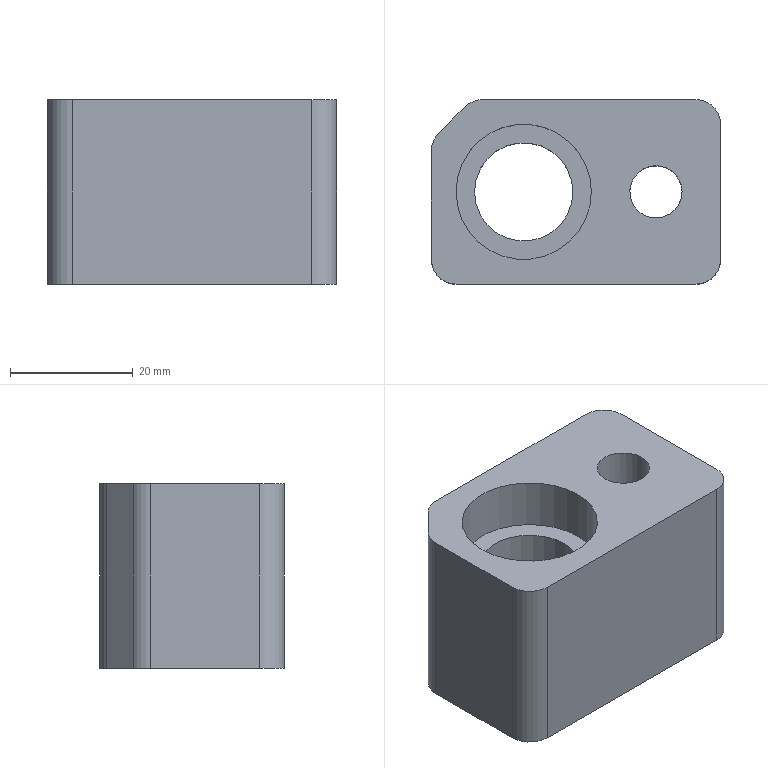Part | NX | features 7 2 | 1 solid | 18 faces | box 47 x 30 x 30 mm | volume 30463 mm3 | plane 9 | cylinder 9 | commonest cylinder face diameters 8 x5 8.5 x1 14.5 x1 16 x1 22 x1
STEP:
#1=CARTESIAN_POINT('',(3123.747,81.578,91.));
#2=VERTEX_POINT('',#1);
#3=CARTESIAN_POINT('',(3123.747,77.328,91.));
#4=DIRECTION('',(0.,0.,-1.));
#5=DIRECTION('',(0.,1.,0.));
#6=AXIS2_PLACEMENT_3D('',#3,#4,#5);
#7=CIRCLE('',#6,4.25);
#8=EDGE_CURVE('',#2,#2,#7,.T.);
#9=ORIENTED_EDGE('',*,*,#8,.T.);
#10=EDGE_LOOP('',(#9));
#11=FACE_BOUND('',#10,.T.);
#12=CARTESIAN_POINT('',(3130.247,62.328,91.));
#13=VERTEX_POINT('',#12);
#14=CARTESIAN_POINT('',(3091.247,62.328,91.));
#15=VERTEX_POINT('',#14);
#16=CARTESIAN_POINT('',(3102.247,62.328,91.));
#17=DIRECTION('',(-1.,0.,0.));
#18=VECTOR('',#17,1000.);
#19=LINE('',#16,#18);
#20=EDGE_CURVE('',#13,#15,#19,.T.);
#21=ORIENTED_EDGE('',*,*,#20,.F.);
#22=CARTESIAN_POINT('',(3134.247,66.328,91.));
#23=VERTEX_POINT('',#22);
#24=CARTESIAN_POINT('',(3130.247,66.328,91.));
#25=DIRECTION('',(0.,0.,1.));
#26=DIRECTION('',(0.,1.,0.));
#27=AXIS2_PLACEMENT_3D('',#24,#25,#26);
#28=CIRCLE('',#27,4.);
#29=EDGE_CURVE('',#13,#23,#28,.T.);
#30=ORIENTED_EDGE('',*,*,#29,.T.);
#31=CARTESIAN_POINT('',(3134.247,88.328,91.));
#32=VERTEX_POINT('',#31);
#33=CARTESIAN_POINT('',(3134.247,77.328,91.));
#34=DIRECTION('',(0.,-1.,0.));
#35=VECTOR('',#34,1000.);
#36=LINE('',#33,#35);
#37=EDGE_CURVE('',#32,#23,#36,.T.);
#38=ORIENTED_EDGE('',*,*,#37,.F.);
#39=CARTESIAN_POINT('',(3130.247,92.328,91.));
#40=VERTEX_POINT('',#39);
#41=CARTESIAN_POINT('',(3130.247,88.328,91.));
#42=DIRECTION('',(0.,0.,1.));
#43=DIRECTION('',(0.,1.,0.));
#44=AXIS2_PLACEMENT_3D('',#41,#42,#43);
#45=CIRCLE('',#44,4.);
#46=EDGE_CURVE('',#32,#40,#45,.T.);
#47=ORIENTED_EDGE('',*,*,#46,.T.);
#48=CARTESIAN_POINT('',(3095.54,92.328,91.));
#49=VERTEX_POINT('',#48);
#50=CARTESIAN_POINT('',(3102.247,92.328,91.));
#51=DIRECTION('',(1.,0.,0.));
#52=VECTOR('',#51,1000.);
#53=LINE('',#50,#52);
#54=EDGE_CURVE('',#49,#40,#53,.T.);
#55=ORIENTED_EDGE('',*,*,#54,.F.);
#56=CARTESIAN_POINT('',(3092.711,91.157,91.));
#57=VERTEX_POINT('',#56);
#58=CARTESIAN_POINT('',(3095.54,88.328,91.));
#59=DIRECTION('',(0.,0.,1.));
#60=DIRECTION('',(0.,1.,0.));
#61=AXIS2_PLACEMENT_3D('',#58,#59,#60);
#62=CIRCLE('',#61,4.);
#63=EDGE_CURVE('',#49,#57,#62,.T.);
#64=ORIENTED_EDGE('',*,*,#63,.T.);
#65=CARTESIAN_POINT('',(3088.419,86.864,91.));
#66=VERTEX_POINT('',#65);
#67=CARTESIAN_POINT('',(3091.815,90.26,91.));
#68=DIRECTION('',(-0.7071,-0.7071,0.));
#69=VECTOR('',#68,1000.);
#70=LINE('',#67,#69);
#71=EDGE_CURVE('',#57,#66,#70,.T.);
#72=ORIENTED_EDGE('',*,*,#71,.T.);
#73=CARTESIAN_POINT('',(3087.247,84.035,91.));
#74=VERTEX_POINT('',#73);
#75=CARTESIAN_POINT('',(3091.247,84.035,91.));
#76=DIRECTION('',(0.,0.,1.));
#77=DIRECTION('',(0.,1.,0.));
#78=AXIS2_PLACEMENT_3D('',#75,#76,#77);
#79=CIRCLE('',#78,4.);
#80=EDGE_CURVE('',#66,#74,#79,.T.);
#81=ORIENTED_EDGE('',*,*,#80,.T.);
#82=CARTESIAN_POINT('',(3087.247,66.328,91.));
#83=VERTEX_POINT('',#82);
#84=CARTESIAN_POINT('',(3087.247,77.328,91.));
#85=DIRECTION('',(0.,1.,0.));
#86=VECTOR('',#85,1000.);
#87=LINE('',#84,#86);
#88=EDGE_CURVE('',#83,#74,#87,.T.);
#89=ORIENTED_EDGE('',*,*,#88,.F.);
#90=CARTESIAN_POINT('',(3091.247,66.328,91.));
#91=DIRECTION('',(0.,0.,1.));
#92=DIRECTION('',(0.,1.,0.));
#93=AXIS2_PLACEMENT_3D('',#90,#91,#92);
#94=CIRCLE('',#93,4.);
#95=EDGE_CURVE('',#83,#15,#94,.T.);
#96=ORIENTED_EDGE('',*,*,#95,.T.);
#97=EDGE_LOOP('',(#21,#30,#38,#47,#55,#64,#72,#81,#89,#96));
#98=FACE_BOUND('',#97,.T.);
#99=CARTESIAN_POINT('',(3113.247,77.328,91.));
#100=VERTEX_POINT('',#99);
#101=CARTESIAN_POINT('',(3102.247,77.328,91.));
#102=DIRECTION('',(0.,0.,1.));
#103=DIRECTION('',(1.,0.,0.));
#104=AXIS2_PLACEMENT_3D('',#101,#102,#103);
#105=CIRCLE('',#104,11.);
#106=EDGE_CURVE('',#100,#100,#105,.T.);
#107=ORIENTED_EDGE('',*,*,#106,.F.);
#108=EDGE_LOOP('',(#107));
#109=FACE_BOUND('',#108,.T.);
#110=CARTESIAN_POINT('',(3104.747,77.328,91.));
#111=DIRECTION('',(0.,0.,1.));
#112=DIRECTION('',(0.,-1.,0.));
#113=AXIS2_PLACEMENT_3D('',#110,#111,#112);
#114=PLANE('',#113);
#115=ADVANCED_FACE('',(#11,#98,#109),#114,.T.);
#116=CARTESIAN_POINT('',(3134.247,66.328,61.));
#117=VERTEX_POINT('',#116);
#118=CARTESIAN_POINT('',(3134.247,88.328,61.));
#119=VERTEX_POINT('',#118);
#120=CARTESIAN_POINT('',(3134.247,-99.672,61.));
#121=DIRECTION('',(0.,1.,0.));
#122=VECTOR('',#121,1000.);
#123=LINE('',#120,#122);
#124=EDGE_CURVE('',#117,#119,#123,.T.);
#125=ORIENTED_EDGE('',*,*,#124,.F.);
#126=CARTESIAN_POINT('',(3130.247,62.328,61.));
#127=VERTEX_POINT('',#126);
#128=CARTESIAN_POINT('',(3130.247,66.328,61.));
#129=DIRECTION('',(0.,0.,-1.));
#130=DIRECTION('',(-1.,0.,0.));
#131=AXIS2_PLACEMENT_3D('',#128,#129,#130);
#132=CIRCLE('',#131,4.);
#133=EDGE_CURVE('',#117,#127,#132,.T.);
#134=ORIENTED_EDGE('',*,*,#133,.T.);
#135=CARTESIAN_POINT('',(3091.247,62.328,61.));
#136=VERTEX_POINT('',#135);
#137=CARTESIAN_POINT('',(3287.247,62.328,61.));
#138=DIRECTION('',(1.,0.,0.));
#139=VECTOR('',#138,1000.);
#140=LINE('',#137,#139);
#141=EDGE_CURVE('',#136,#127,#140,.T.);
#142=ORIENTED_EDGE('',*,*,#141,.F.);
#143=CARTESIAN_POINT('',(3087.247,66.328,61.));
#144=VERTEX_POINT('',#143);
#145=CARTESIAN_POINT('',(3091.247,66.328,61.));
#146=DIRECTION('',(0.,0.,-1.));
#147=DIRECTION('',(-1.,0.,0.));
#148=AXIS2_PLACEMENT_3D('',#145,#146,#147);
#149=CIRCLE('',#148,4.);
#150=EDGE_CURVE('',#136,#144,#149,.T.);
#151=ORIENTED_EDGE('',*,*,#150,.T.);
#152=CARTESIAN_POINT('',(3087.247,84.035,61.));
#153=VERTEX_POINT('',#152);
#154=CARTESIAN_POINT('',(3087.247,-99.672,61.));
#155=DIRECTION('',(0.,-1.,0.));
#156=VECTOR('',#155,1000.);
#157=LINE('',#154,#156);
#158=EDGE_CURVE('',#153,#144,#157,.T.);
#159=ORIENTED_EDGE('',*,*,#158,.F.);
#160=CARTESIAN_POINT('',(3088.419,86.864,61.));
#161=VERTEX_POINT('',#160);
#162=CARTESIAN_POINT('',(3091.247,84.035,61.));
#163=DIRECTION('',(0.,0.,-1.));
#164=DIRECTION('',(-1.,0.,0.));
#165=AXIS2_PLACEMENT_3D('',#162,#163,#164);
#166=CIRCLE('',#165,4.);
#167=EDGE_CURVE('',#153,#161,#166,.T.);
#168=ORIENTED_EDGE('',*,*,#167,.T.);
#169=CARTESIAN_POINT('',(3092.711,91.157,61.));
#170=VERTEX_POINT('',#169);
#171=CARTESIAN_POINT('',(3094.565,93.01,61.));
#172=DIRECTION('',(0.7071,0.7071,0.));
#173=VECTOR('',#172,1000.);
#174=LINE('',#171,#173);
#175=EDGE_CURVE('',#161,#170,#174,.T.);
#176=ORIENTED_EDGE('',*,*,#175,.T.);
#177=CARTESIAN_POINT('',(3095.54,92.328,61.));
#178=VERTEX_POINT('',#177);
#179=CARTESIAN_POINT('',(3095.54,88.328,61.));
#180=DIRECTION('',(0.,0.,-1.));
#181=DIRECTION('',(-1.,0.,0.));
#182=AXIS2_PLACEMENT_3D('',#179,#180,#181);
#183=CIRCLE('',#182,4.);
#184=EDGE_CURVE('',#170,#178,#183,.T.);
#185=ORIENTED_EDGE('',*,*,#184,.T.);
#186=CARTESIAN_POINT('',(3130.247,92.328,61.));
#187=VERTEX_POINT('',#186);
#188=CARTESIAN_POINT('',(3287.247,92.328,61.));
#189=DIRECTION('',(-1.,0.,0.));
#190=VECTOR('',#189,1000.);
#191=LINE('',#188,#190);
#192=EDGE_CURVE('',#187,#178,#191,.T.);
#193=ORIENTED_EDGE('',*,*,#192,.F.);
#194=CARTESIAN_POINT('',(3130.247,88.328,61.));
#195=DIRECTION('',(0.,0.,-1.));
#196=DIRECTION('',(-1.,0.,0.));
#197=AXIS2_PLACEMENT_3D('',#194,#195,#196);
#198=CIRCLE('',#197,4.);
#199=EDGE_CURVE('',#187,#119,#198,.T.);
#200=ORIENTED_EDGE('',*,*,#199,.T.);
#201=EDGE_LOOP('',(#125,#134,#142,#151,#159,#168,#176,#185,#193,#200));
#202=FACE_BOUND('',#201,.T.);
#203=CARTESIAN_POINT('',(3116.497,77.328,61.));
#204=VERTEX_POINT('',#203);
#205=CARTESIAN_POINT('',(3123.747,77.328,61.));
#206=DIRECTION('',(0.,0.,-1.));
#207=DIRECTION('',(-1.,0.,0.));
#208=AXIS2_PLACEMENT_3D('',#205,#206,#207);
#209=CIRCLE('',#208,7.25);
#210=EDGE_CURVE('',#204,#204,#209,.T.);
#211=ORIENTED_EDGE('',*,*,#210,.F.);
#212=EDGE_LOOP('',(#211));
#213=FACE_BOUND('',#212,.T.);
#214=CARTESIAN_POINT('',(3094.247,77.328,61.));
#215=VERTEX_POINT('',#214);
#216=CARTESIAN_POINT('',(3102.247,77.328,61.));
#217=DIRECTION('',(0.,0.,1.));
#218=DIRECTION('',(-1.,0.,0.));
#219=AXIS2_PLACEMENT_3D('',#216,#217,#218);
#220=CIRCLE('',#219,8.);
#221=EDGE_CURVE('',#215,#215,#220,.T.);
#222=ORIENTED_EDGE('',*,*,#221,.T.);
#223=EDGE_LOOP('',(#222));
#224=FACE_BOUND('',#223,.T.);
#225=CARTESIAN_POINT('',(3287.247,-99.672,61.));
#226=DIRECTION('',(0.,0.,-1.));
#227=DIRECTION('',(0.,1.,0.));
#228=AXIS2_PLACEMENT_3D('',#225,#226,#227);
#229=PLANE('',#228);
#230=ADVANCED_FACE('',(#202,#213,#224),#229,.T.);
#231=ORIENTED_EDGE('',*,*,#88,.T.);
#232=CARTESIAN_POINT('',(3087.247,84.035,-5.));
#233=DIRECTION('',(0.,0.,-1.));
#234=VECTOR('',#233,1000.);
#235=LINE('',#232,#234);
#236=EDGE_CURVE('',#74,#153,#235,.T.);
#237=ORIENTED_EDGE('',*,*,#236,.T.);
#238=ORIENTED_EDGE('',*,*,#158,.T.);
#239=CARTESIAN_POINT('',(3087.247,66.328,-5.));
#240=DIRECTION('',(0.,0.,1.));
#241=VECTOR('',#240,1000.);
#242=LINE('',#239,#241);
#243=EDGE_CURVE('',#144,#83,#242,.T.);
#244=ORIENTED_EDGE('',*,*,#243,.T.);
#245=EDGE_LOOP('',(#231,#237,#238,#244));
#246=FACE_BOUND('',#245,.T.);
#247=CARTESIAN_POINT('',(3087.247,77.328,-5.));
#248=DIRECTION('',(-1.,0.,0.));
#249=DIRECTION('',(0.,0.,-1.));
#250=AXIS2_PLACEMENT_3D('',#247,#248,#249);
#251=PLANE('',#250);
#252=ADVANCED_FACE('',(#246),#251,.T.);
#253=ORIENTED_EDGE('',*,*,#54,.T.);
#254=CARTESIAN_POINT('',(3130.247,92.328,-5.));
#255=DIRECTION('',(0.,0.,-1.));
#256=VECTOR('',#255,1000.);
#257=LINE('',#254,#256);
#258=EDGE_CURVE('',#40,#187,#257,.T.);
#259=ORIENTED_EDGE('',*,*,#258,.T.);
#260=ORIENTED_EDGE('',*,*,#192,.T.);
#261=CARTESIAN_POINT('',(3095.54,92.328,-5.));
#262=DIRECTION('',(0.,0.,1.));
#263=VECTOR('',#262,1000.);
#264=LINE('',#261,#263);
#265=EDGE_CURVE('',#178,#49,#264,.T.);
#266=ORIENTED_EDGE('',*,*,#265,.T.);
#267=EDGE_LOOP('',(#253,#259,#260,#266));
#268=FACE_BOUND('',#267,.T.);
#269=CARTESIAN_POINT('',(3102.247,92.328,-5.));
#270=DIRECTION('',(0.,1.,0.));
#271=DIRECTION('',(0.,0.,1.));
#272=AXIS2_PLACEMENT_3D('',#269,#270,#271);
#273=PLANE('',#272);
#274=ADVANCED_FACE('',(#268),#273,.T.);
#275=ORIENTED_EDGE('',*,*,#37,.T.);
#276=CARTESIAN_POINT('',(3134.247,66.328,-5.));
#277=DIRECTION('',(0.,0.,-1.));
#278=VECTOR('',#277,1000.);
#279=LINE('',#276,#278);
#280=EDGE_CURVE('',#23,#117,#279,.T.);
#281=ORIENTED_EDGE('',*,*,#280,.T.);
#282=ORIENTED_EDGE('',*,*,#124,.T.);
#283=CARTESIAN_POINT('',(3134.247,88.328,-5.));
#284=DIRECTION('',(0.,0.,1.));
#285=VECTOR('',#284,1000.);
#286=LINE('',#283,#285);
#287=EDGE_CURVE('',#119,#32,#286,.T.);
#288=ORIENTED_EDGE('',*,*,#287,.T.);
#289=EDGE_LOOP('',(#275,#281,#282,#288));
#290=FACE_BOUND('',#289,.T.);
#291=CARTESIAN_POINT('',(3134.247,77.328,-5.));
#292=DIRECTION('',(1.,0.,0.));
#293=DIRECTION('',(0.,0.,1.));
#294=AXIS2_PLACEMENT_3D('',#291,#292,#293);
#295=PLANE('',#294);
#296=ADVANCED_FACE('',(#290),#295,.T.);
#297=ORIENTED_EDGE('',*,*,#141,.T.);
#298=CARTESIAN_POINT('',(3130.247,62.328,-5.));
#299=DIRECTION('',(0.,0.,1.));
#300=VECTOR('',#299,1000.);
#301=LINE('',#298,#300);
#302=EDGE_CURVE('',#127,#13,#301,.T.);
#303=ORIENTED_EDGE('',*,*,#302,.T.);
#304=ORIENTED_EDGE('',*,*,#20,.T.);
#305=CARTESIAN_POINT('',(3091.247,62.328,-5.));
#306=DIRECTION('',(0.,0.,-1.));
#307=VECTOR('',#306,1000.);
#308=LINE('',#305,#307);
#309=EDGE_CURVE('',#15,#136,#308,.T.);
#310=ORIENTED_EDGE('',*,*,#309,.T.);
#311=EDGE_LOOP('',(#297,#303,#304,#310));
#312=FACE_BOUND('',#311,.T.);
#313=CARTESIAN_POINT('',(3102.247,62.328,-5.));
#314=DIRECTION('',(0.,-1.,0.));
#315=DIRECTION('',(0.,0.,-1.));
#316=AXIS2_PLACEMENT_3D('',#313,#314,#315);
#317=PLANE('',#316);
#318=ADVANCED_FACE('',(#312),#317,.T.);
#319=ORIENTED_EDGE('',*,*,#71,.F.);
#320=CARTESIAN_POINT('',(3092.711,91.157,-5.));
#321=DIRECTION('',(0.,0.,-1.));
#322=VECTOR('',#321,1000.);
#323=LINE('',#320,#322);
#324=EDGE_CURVE('',#57,#170,#323,.T.);
#325=ORIENTED_EDGE('',*,*,#324,.T.);
#326=ORIENTED_EDGE('',*,*,#175,.F.);
#327=CARTESIAN_POINT('',(3088.419,86.864,-5.));
#328=DIRECTION('',(0.,0.,1.));
#329=VECTOR('',#328,1000.);
#330=LINE('',#327,#329);
#331=EDGE_CURVE('',#161,#66,#330,.T.);
#332=ORIENTED_EDGE('',*,*,#331,.T.);
#333=EDGE_LOOP('',(#319,#325,#326,#332));
#334=FACE_BOUND('',#333,.T.);
#335=CARTESIAN_POINT('',(3094.565,93.01,-5.));
#336=DIRECTION('',(0.7071,-0.7071,0.));
#337=DIRECTION('',(0.,0.,1.));
#338=AXIS2_PLACEMENT_3D('',#335,#336,#337);
#339=PLANE('',#338);
#340=ADVANCED_FACE('',(#334),#339,.F.);
#341=ORIENTED_EDGE('',*,*,#133,.F.);
#342=ORIENTED_EDGE('',*,*,#280,.F.);
#343=ORIENTED_EDGE('',*,*,#29,.F.);
#344=ORIENTED_EDGE('',*,*,#302,.F.);
#345=EDGE_LOOP('',(#341,#342,#343,#344));
#346=FACE_BOUND('',#345,.T.);
#347=CARTESIAN_POINT('',(3130.247,66.328,-5.));
#348=DIRECTION('',(0.,0.,-1.));
#349=DIRECTION('',(0.,-1.,0.));
#350=AXIS2_PLACEMENT_3D('',#347,#348,#349);
#351=CYLINDRICAL_SURFACE('',#350,4.);
#352=ADVANCED_FACE('',(#346),#351,.T.);
#353=ORIENTED_EDGE('',*,*,#199,.F.);
#354=ORIENTED_EDGE('',*,*,#258,.F.);
#355=ORIENTED_EDGE('',*,*,#46,.F.);
#356=ORIENTED_EDGE('',*,*,#287,.F.);
#357=EDGE_LOOP('',(#353,#354,#355,#356));
#358=FACE_BOUND('',#357,.T.);
#359=CARTESIAN_POINT('',(3130.247,88.328,-5.));
#360=DIRECTION('',(0.,0.,-1.));
#361=DIRECTION('',(0.,-1.,0.));
#362=AXIS2_PLACEMENT_3D('',#359,#360,#361);
#363=CYLINDRICAL_SURFACE('',#362,4.);
#364=ADVANCED_FACE('',(#358),#363,.T.);
#365=ORIENTED_EDGE('',*,*,#184,.F.);
#366=ORIENTED_EDGE('',*,*,#324,.F.);
#367=ORIENTED_EDGE('',*,*,#63,.F.);
#368=ORIENTED_EDGE('',*,*,#265,.F.);
#369=EDGE_LOOP('',(#365,#366,#367,#368));
#370=FACE_BOUND('',#369,.T.);
#371=CARTESIAN_POINT('',(3095.54,88.328,-5.));
#372=DIRECTION('',(0.,0.,1.));
#373=DIRECTION('',(0.,1.,0.));
#374=AXIS2_PLACEMENT_3D('',#371,#372,#373);
#375=CYLINDRICAL_SURFACE('',#374,4.);
#376=ADVANCED_FACE('',(#370),#375,.T.);
#377=ORIENTED_EDGE('',*,*,#80,.F.);
#378=ORIENTED_EDGE('',*,*,#331,.F.);
#379=ORIENTED_EDGE('',*,*,#167,.F.);
#380=ORIENTED_EDGE('',*,*,#236,.F.);
#381=EDGE_LOOP('',(#377,#378,#379,#380));
#382=FACE_BOUND('',#381,.T.);
#383=CARTESIAN_POINT('',(3091.247,84.035,-5.));
#384=DIRECTION('',(0.,0.,-1.));
#385=DIRECTION('',(0.,-1.,0.));
#386=AXIS2_PLACEMENT_3D('',#383,#384,#385);
#387=CYLINDRICAL_SURFACE('',#386,4.);
#388=ADVANCED_FACE('',(#382),#387,.T.);
#389=ORIENTED_EDGE('',*,*,#150,.F.);
#390=ORIENTED_EDGE('',*,*,#309,.F.);
#391=ORIENTED_EDGE('',*,*,#95,.F.);
#392=ORIENTED_EDGE('',*,*,#243,.F.);
#393=EDGE_LOOP('',(#389,#390,#391,#392));
#394=FACE_BOUND('',#393,.T.);
#395=CARTESIAN_POINT('',(3091.247,66.328,-5.));
#396=DIRECTION('',(0.,0.,-1.));
#397=DIRECTION('',(0.,-1.,0.));
#398=AXIS2_PLACEMENT_3D('',#395,#396,#397);
#399=CYLINDRICAL_SURFACE('',#398,4.);
#400=ADVANCED_FACE('',(#394),#399,.T.);
#401=CARTESIAN_POINT('',(3127.997,77.328,76.));
#402=VERTEX_POINT('',#401);
#403=CARTESIAN_POINT('',(3123.747,77.328,76.));
#404=DIRECTION('',(0.,0.,1.));
#405=DIRECTION('',(1.,0.,0.));
#406=AXIS2_PLACEMENT_3D('',#403,#404,#405);
#407=CIRCLE('',#406,4.25);
#408=EDGE_CURVE('',#402,#402,#407,.T.);
#409=ORIENTED_EDGE('',*,*,#408,.F.);
#410=EDGE_LOOP('',(#409));
#411=FACE_BOUND('',#410,.T.);
#412=ORIENTED_EDGE('',*,*,#8,.F.);
#413=EDGE_LOOP('',(#412));
#414=FACE_BOUND('',#413,.T.);
#415=CARTESIAN_POINT('',(3123.747,77.328,55.));
#416=DIRECTION('',(0.,0.,1.));
#417=DIRECTION('',(0.,-1.,0.));
#418=AXIS2_PLACEMENT_3D('',#415,#416,#417);
#419=CYLINDRICAL_SURFACE('',#418,4.25);
#420=ADVANCED_FACE('',(#411,#414),#419,.F.);
#421=ORIENTED_EDGE('',*,*,#408,.T.);
#422=EDGE_LOOP('',(#421));
#423=FACE_BOUND('',#422,.T.);
#424=CARTESIAN_POINT('',(3130.997,77.328,76.));
#425=VERTEX_POINT('',#424);
#426=CARTESIAN_POINT('',(3123.747,77.328,76.));
#427=DIRECTION('',(0.,0.,1.));
#428=DIRECTION('',(1.,0.,0.));
#429=AXIS2_PLACEMENT_3D('',#426,#427,#428);
#430=CIRCLE('',#429,7.25);
#431=EDGE_CURVE('',#425,#425,#430,.T.);
#432=ORIENTED_EDGE('',*,*,#431,.F.);
#433=EDGE_LOOP('',(#432));
#434=FACE_BOUND('',#433,.T.);
#435=CARTESIAN_POINT('',(3123.747,77.328,76.));
#436=DIRECTION('',(0.,0.,1.));
#437=DIRECTION('',(0.,-1.,0.));
#438=AXIS2_PLACEMENT_3D('',#435,#436,#437);
#439=PLANE('',#438);
#440=ADVANCED_FACE('',(#423,#434),#439,.F.);
#441=ORIENTED_EDGE('',*,*,#210,.T.);
#442=EDGE_LOOP('',(#441));
#443=FACE_BOUND('',#442,.T.);
#444=ORIENTED_EDGE('',*,*,#431,.T.);
#445=EDGE_LOOP('',(#444));
#446=FACE_BOUND('',#445,.T.);
#447=CARTESIAN_POINT('',(3123.747,77.328,55.));
#448=DIRECTION('',(0.,0.,1.));
#449=DIRECTION('',(0.,-1.,0.));
#450=AXIS2_PLACEMENT_3D('',#447,#448,#449);
#451=CYLINDRICAL_SURFACE('',#450,7.25);
#452=ADVANCED_FACE('',(#443,#446),#451,.F.);
#453=ORIENTED_EDGE('',*,*,#221,.F.);
#454=EDGE_LOOP('',(#453));
#455=FACE_BOUND('',#454,.T.);
#456=CARTESIAN_POINT('',(3094.247,77.328,82.7));
#457=VERTEX_POINT('',#456);
#458=CARTESIAN_POINT('',(3102.247,77.328,82.7));
#459=DIRECTION('',(0.,0.,-1.));
#460=DIRECTION('',(-1.,0.,0.));
#461=AXIS2_PLACEMENT_3D('',#458,#459,#460);
#462=CIRCLE('',#461,8.);
#463=EDGE_CURVE('',#457,#457,#462,.T.);
#464=ORIENTED_EDGE('',*,*,#463,.F.);
#465=EDGE_LOOP('',(#464));
#466=FACE_BOUND('',#465,.T.);
#467=CARTESIAN_POINT('',(3102.247,77.328,44.5));
#468=DIRECTION('',(0.,0.,-1.));
#469=DIRECTION('',(-1.,0.,0.));
#470=AXIS2_PLACEMENT_3D('',#467,#468,#469);
#471=CYLINDRICAL_SURFACE('',#470,8.);
#472=ADVANCED_FACE('',(#455,#466),#471,.F.);
#473=CARTESIAN_POINT('',(3091.247,77.328,82.7));
#474=VERTEX_POINT('',#473);
#475=CARTESIAN_POINT('',(3102.247,77.328,82.7));
#476=DIRECTION('',(0.,0.,-1.));
#477=DIRECTION('',(-1.,0.,0.));
#478=AXIS2_PLACEMENT_3D('',#475,#476,#477);
#479=CIRCLE('',#478,11.);
#480=EDGE_CURVE('',#474,#474,#479,.T.);
#481=ORIENTED_EDGE('',*,*,#480,.F.);
#482=EDGE_LOOP('',(#481));
#483=FACE_BOUND('',#482,.T.);
#484=ORIENTED_EDGE('',*,*,#463,.T.);
#485=EDGE_LOOP('',(#484));
#486=FACE_BOUND('',#485,.T.);
#487=CARTESIAN_POINT('',(3102.247,77.328,82.7));
#488=DIRECTION('',(0.,0.,-1.));
#489=DIRECTION('',(-1.,0.,0.));
#490=AXIS2_PLACEMENT_3D('',#487,#488,#489);
#491=PLANE('',#490);
#492=ADVANCED_FACE('',(#483,#486),#491,.F.);
#493=ORIENTED_EDGE('',*,*,#480,.T.);
#494=EDGE_LOOP('',(#493));
#495=FACE_BOUND('',#494,.T.);
#496=ORIENTED_EDGE('',*,*,#106,.T.);
#497=EDGE_LOOP('',(#496));
#498=FACE_BOUND('',#497,.T.);
#499=CARTESIAN_POINT('',(3102.247,77.328,87.));
#500=DIRECTION('',(0.,0.,-1.));
#501=DIRECTION('',(-1.,0.,0.));
#502=AXIS2_PLACEMENT_3D('',#499,#500,#501);
#503=CYLINDRICAL_SURFACE('',#502,11.);
#504=ADVANCED_FACE('',(#495,#498),#503,.F.);
#505=CLOSED_SHELL('',(#115,#230,#252,#274,#296,#318,#340,#352,#364,#376,#388,#400,#420,#440,#452,#472,#492,#504));
#506=MANIFOLD_SOLID_BREP('',#505);
#507=(LENGTH_UNIT()NAMED_UNIT(*)SI_UNIT(.MILLI.,.METRE.));
#508=UNCERTAINTY_MEASURE_WITH_UNIT(LENGTH_MEASURE(0.00001),#507,'','');
#509=(NAMED_UNIT(*)PLANE_ANGLE_UNIT()SI_UNIT($,.RADIAN.));
#510=(NAMED_UNIT(*)SI_UNIT($,.STERADIAN.)SOLID_ANGLE_UNIT());
#511=(GEOMETRIC_REPRESENTATION_CONTEXT(3)GLOBAL_UNCERTAINTY_ASSIGNED_CONTEXT((#508))GLOBAL_UNIT_ASSIGNED_CONTEXT((#507,#509,#510))REPRESENTATION_CONTEXT('',''));
#512=ADVANCED_BREP_SHAPE_REPRESENTATION('',(#506),#511);